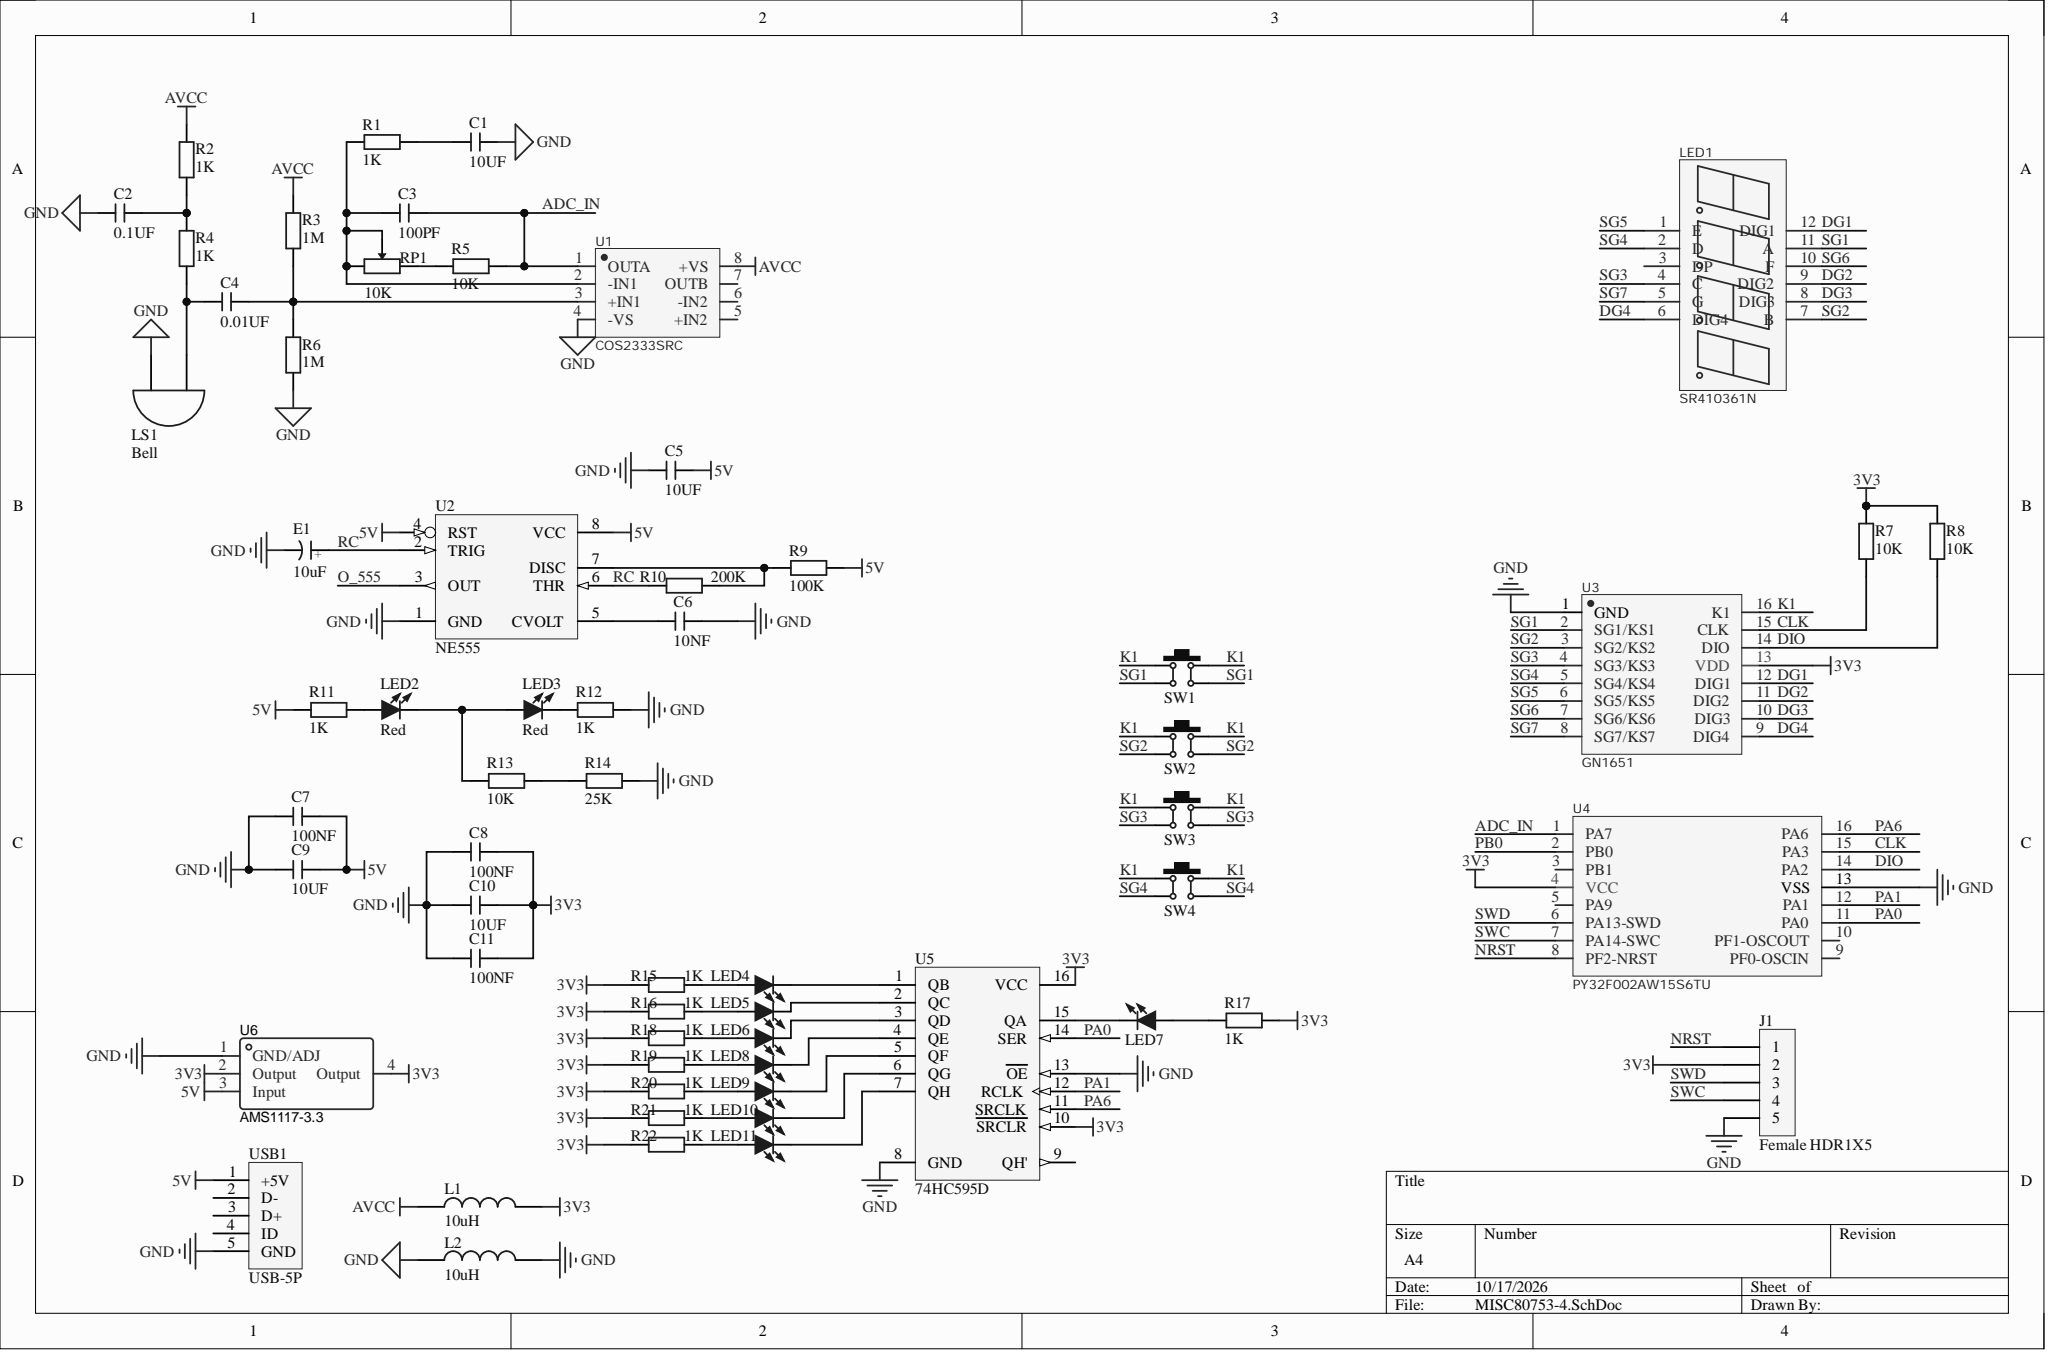Circuit board | Altium Designer | 61 parts | 54 nets
Bill of materials:
Comment,Description,Designator,Footprint,LibRef,Quantity
"10UF","Chip capacitor","C1, C5, C9, C10","C 0805_L","C","4"
"0.1UF","Chip capacitor","C2","C 0805_L","C","1"
"100PF","Chip capacitor","C3","C 0805_L","C","1"
"0.01UF","Chip capacitor","C4","C 0805_L","C","1"
"10NF","Chip capacitor","C6","C 0805_L","C","1"
"100NF","Chip capacitor","C7, C8, C11","C 0805_L","C","3"
"10uF","Chip electrolytic capacitor","E1","CM A(3*5.4)","CE_SMD","1"
"Female HDR1X5","","J1","Fe-HDR1X5/2.54-S","Female HDR1X5","1"
"10uH","Low-power chip inductor","L1, L2","L 0805","L","2"
"SR410361N","","LED1","LED-SEG-TH_12P-L30.0-W14.0-P2.54-S10.26-BL","SR410361N","1"
"Red","Chip LED","LED2, LED3, LED4, LED5, LED6, LED7, LED8, LED9, LED10, LED11","LED 0805G","LED-SMD","10"
"Bell","Electrical Bell","LS1","PIN2","Bell","1"
"1K","Chip resistor","R1, R2, R4, R11, R12, R15, R16, R17, R18, R19, R20, R21, R22","R 0805_L","R","13"
"1M","Chip resistor","R3, R6","R 0805_L","R","2"
"10K","Chip resistor","R5, R7, R8, R13","R 0805_L","R","4"
"100K","Chip resistor","R9","R 0805_L","R","1"
"200K","Chip resistor","R10","R 0805_L","R","1"
"25K","Chip resistor","R14","R 0805_L","R","1"
"10K","Single-gang potentiometer","RP1","3296W","RP","1"
"6x6x5","Through-hole 6x6 tactile switch","SW1, SW2, SW3, SW4","四脚轻触开关","TSW DIP-6x6","4"
"COS2333SRC","","U1","SOP-8_L4.9-W3.9-P1.27-LS6.0-BL","COS2333SRC","1"
"NE555","General-Purpose Single Bipolar Timer","U2","SOP8","NE555D","1"
"GN1651","","U3","SOP-16_L9.9-W3.9-P1.27-LS6.1-BL","GN1651","1"
"PY32F002AW15S6TU","","U4","SOP-16_L9.9-W3.9-P1.27-LS6.0-BL","PY32F002AW15S6TU","1"
"74HC595D","8-Bit Shift Register with 3-State Output Registers","U5","SOP16","SN74HC595D","1"
"AMS1117-3.3","","U6","AMS1117-3.3","AMS1117-3.3","1"
"USB-5P","Micro USB female socket","USB1","USB-MICRO_A","USB-5P","1"
Netlist (Protel format):
[
C1
C 0805_L
10UF



]
[
C2
C 0805_L
0.1UF



]
[
C3
C 0805_L
100PF



]
[
C4
C 0805_L
0.01UF



]
[
C5
C 0805_L
10UF



]
[
C6
C 0805_L
10NF



]
[
C7
C 0805_L
100NF



]
[
C8
C 0805_L
100NF



]
[
C9
C 0805_L
10UF



]
[
C10
C 0805_L
10UF



]
[
C11
C 0805_L
100NF



]
[
E1
CM A(3*5.4)
10uF



]
[
J1
Fe-HDR1X5/2.54-S
Female HDR1X5



]
[
L1
L 0805
10uH



]
[
L2
L 0805
10uH



]
[
LED1
LED-SEG-TH_12P-L30.0-W14.0-P2.54-S10.26-BL
SR410361N



]
[
LED2
LED 0805G
Red



]
[
LED3
LED 0805G
Red



]
[
LED4
LED 0805G
Red



]
[
LED5
LED 0805G
Red



]
[
LED6
LED 0805G
Red



]
[
LED7
LED 0805G
Red



]
[
LED8
LED 0805G
Red



]
[
LED9
LED 0805G
Red



]
[
LED10
LED 0805G
Red



]
[
LED11
LED 0805G
Red



]
[
LS1
PIN2
Bell



]
[
R1
R 0805_L
1K



]
[
R2
R 0805_L
1K



]
[
R3
R 0805_L
1M



]
[
R4
R 0805_L
1K



]
[
R5
R 0805_L
10K



]
[
R6
R 0805_L
1M



]
[
R7
R 0805_L
10K



]
[
R8
R 0805_L
10K



]
[
R9
R 0805_L
100K



]
[
R10
R 0805_L
200K



]
[
R11
R 0805_L
1K



]
[
R12
R 0805_L
1K



]
[
R13
R 0805_L
10K



]
[
R14
R 0805_L
25K



]
[
R15
R 0805_L
1K



]
[
R16
R 0805_L
1K



]
[
R17
R 0805_L
1K



]
[
R18
R 0805_L
1K



]
[
R19
R 0805_L
1K



]
[
R20
R 0805_L
1K



]
[
R21
R 0805_L
1K



]
[
R22
R 0805_L
1K



]
[
RP1
3296W
10K



]
[
SW1
四脚轻触开关
6x6x5



]
[
SW2
四脚轻触开关
6x6x5



]
[
SW3
四脚轻触开关
6x6x5



]
[
SW4
四脚轻触开关
6x6x5



]
[
U1
SOP-8_L4.9-W3.9-P1.27-LS6.0-BL
COS2333SRC



]
[
U2
SOP8
NE555



]
[
U3
SOP-16_L9.9-W3.9-P1.27-LS6.1-BL
GN1651



]
[
U4
SOP-16_L9.9-W3.9-P1.27-LS6.0-BL
PY32F002AW15S6TU



]
[
U5
SOP16
74HC595D



]
[
U6
AMS1117-3.3
AMS1117-3.3



]
[
USB1
USB-MICRO_A
USB-5P



]
(
SWD
J1-3
U4-6
)
(
SWC
J1-4
U4-7
)
(
SG7
LED1-5
U3-8
)
(
SG6
LED1-10
U3-7
)
(
SG5
LED1-1
U3-6
)
(
SG4
LED1-2
SW4-3
SW4-4
U3-5
)
(
SG3
LED1-4
SW3-3
SW3-4
U3-4
)
(
SG2
LED1-7
SW2-3
SW2-4
U3-3
)
(
SG1
LED1-11
SW1-3
SW1-4
U3-2
)
(
RC
E1-1
R10-1
U2-2
U2-6
)
(
PA6
U4-16
U5-11
)
(
PA1
U4-12
U5-12
)
(
PA0
U4-11
U5-14
)
(
NRST
J1-1
U4-8
)
(
NetR13_2
R13-2
R14-1
)
(
NetR9_1
R9-1
R10-2
U2-7
)
(
NetR5_1
R5-1
RP1-3
)
(
NetLED11_2
LED11-2
U5-7
)
(
NetLED11_1
LED11-1
R22-2
)
(
NetLED10_2
LED10-2
U5-6
)
(
NetLED10_1
LED10-1
R21-2
)
(
NetLED9_2
LED9-2
U5-5
)
(
NetLED9_1
LED9-1
R20-2
)
(
NetLED8_2
LED8-2
U5-4
)
(
NetLED8_1
LED8-1
R19-2
)
(
NetLED7_2
LED7-2
U5-15
)
(
NetLED7_1
LED7-1
R17-2
)
(
NetLED6_2
LED6-2
U5-3
)
(
NetLED6_1
LED6-1
R18-2
)
(
NetLED5_2
LED5-2
U5-2
)
(
NetLED5_1
LED5-1
R16-2
)
(
NetLED4_2
LED4-2
U5-1
)
(
NetLED4_1
LED4-1
R15-2
)
(
NetLED3_2
LED3-2
R12-1
)
(
NetLED2_2
LED2-2
LED3-1
R13-1
)
(
NetLED2_1
LED2-1
R11-2
)
(
NetC6_1
C6-1
U2-5
)
(
NetC4_2
C4-2
R3-1
R6-1
U1-3
)
(
NetC4_1
C4-1
LS1-1
R4-1
)
(
NetC3_1
C3-1
R1-1
RP1-1
RP1-2
U1-2
)
(
NetC2_2
C2-2
R2-1
R4-2
)
(
NetC1_1
C1-1
R1-2
)
(
K1
SW1-1
SW1-2
SW2-1
SW2-2
SW3-1
SW3-2
SW4-1
SW4-2
U3-16
)
(
GND
C1-2
C2-1
C5-1
C6-2
C7-1
C8-1
C9-1
C10-1
C11-1
E1-2
J1-5
L2-1
L2-2
LS1-2
R6-2
R12-2
R14-2
U1-4
U2-1
U3-1
U4-13
U5-8
U5-13
U6-1
USB1-5
)
(
DIO
R8-1
U3-14
U4-14
)
(
DG4
LED1-6
U3-9
)
(
DG3
LED1-8
U3-10
)
(
DG2
LED1-9
U3-11
)
(
DG1
LED1-12
U3-12
)
(
CLK
R7-1
U3-15
U4-15
)
(
AVCC
L1-1
R2-2
R3-2
U1-8
)
(
ADC_IN
C3-2
R5-2
U1-1
U4-1
)
(
5V
C5-2
C7-2
C9-2
R9-2
R11-1
U2-4
U2-8
U6-3
USB1-1
)
(
3V3
C8-2
C10-2
C11-2
J1-2
L1-2
R7-2
R8-2
R15-1
R16-1
R17-1
R18-1
R19-1
R20-1
R21-1
R22-1
U3-13
U4-4
U5-10
U5-16
U6-2
U6-4
)